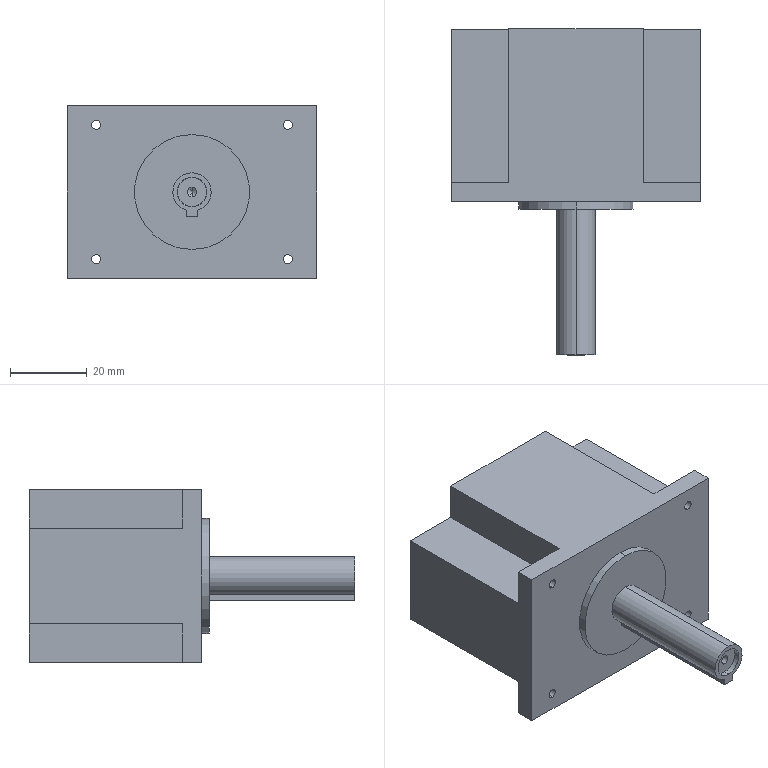Part | SolidWorks | features ICE 4, HoleWzd 2, Extrusion 1 | 1 solid | 64 faces | box 65 x 85 x 45 mm | volume 111801 mm3 | plane 28 | cylinder 24 | cone 12 | commonest cylinder face diameters 2.4 x10 7.619 x10 10 x2 30 x2